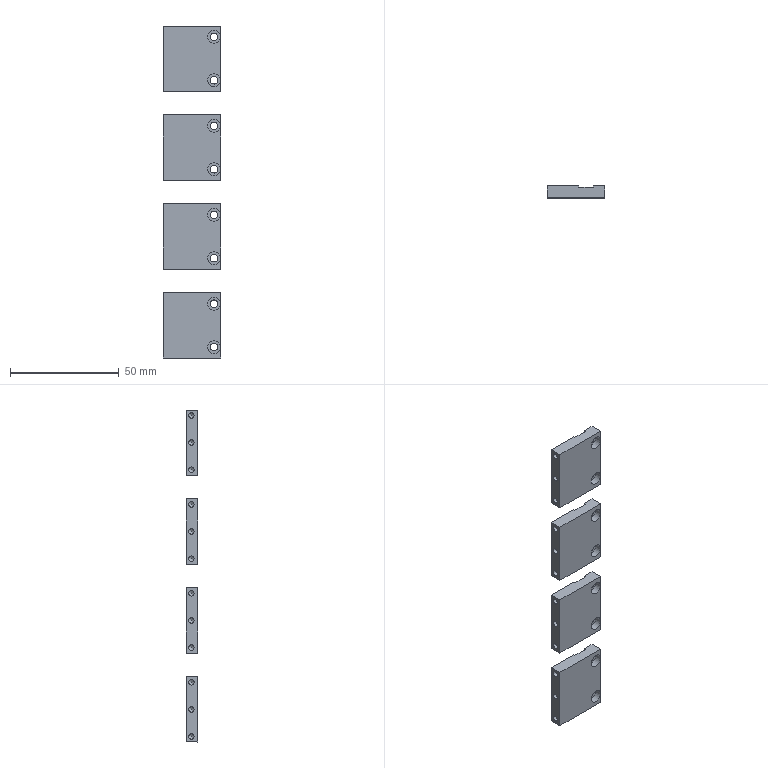Part | 4 solids | 88 faces | box 26.5 x 5.5 x 153 mm | volume 15453 mm3 | plane 48 | cylinder 28 | cone 12 | commonest cylinder face diameters 2.5 x12 3.5 x8 6 x8